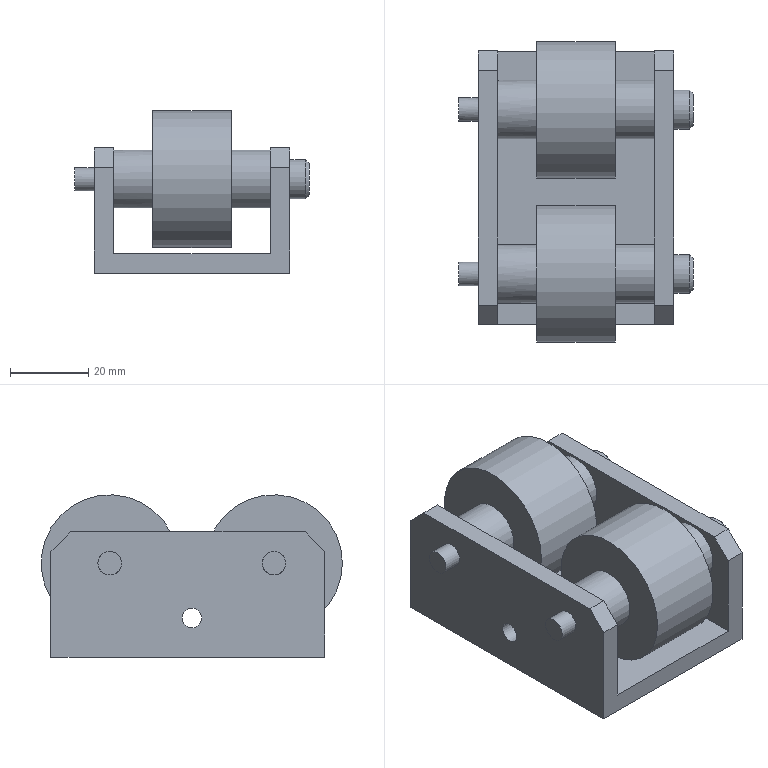Part | NX | features solid 2 | 1 solid | 36 faces | box 60 x 77 x 41.5 mm | volume 82546 mm3 | plane 22 | cylinder 12 | cone 2 | commonest cylinder face diameters 15 x4 5 x2 6 x2 10 x2 35 x2
STEP:
#1=CARTESIAN_POINT('',(200.,655.5,-126.));
#2=VERTEX_POINT('',#1);
#3=CARTESIAN_POINT('',(200.,673.,-126.));
#4=DIRECTION('',(1.,0.,0.));
#5=DIRECTION('',(0.,-1.,0.));
#6=AXIS2_PLACEMENT_3D('',#3,#4,#5);
#7=CIRCLE('',#6,17.5);
#8=EDGE_CURVE('',#2,#2,#7,.T.);
#9=ORIENTED_EDGE('',*,*,#8,.F.);
#10=EDGE_LOOP('',(#9));
#11=FACE_BOUND('',#10,.T.);
#12=CARTESIAN_POINT('',(180.,655.5,-126.));
#13=VERTEX_POINT('',#12);
#14=CARTESIAN_POINT('',(180.,673.,-126.));
#15=DIRECTION('',(1.,0.,0.));
#16=DIRECTION('',(0.,-1.,0.));
#17=AXIS2_PLACEMENT_3D('',#14,#15,#16);
#18=CIRCLE('',#17,17.5);
#19=EDGE_CURVE('',#13,#13,#18,.T.);
#20=ORIENTED_EDGE('',*,*,#19,.T.);
#21=EDGE_LOOP('',(#20));
#22=FACE_BOUND('',#21,.T.);
#23=CARTESIAN_POINT('',(180.,673.,-126.));
#24=DIRECTION('',(1.,0.,0.));
#25=DIRECTION('',(0.,0.,-1.));
#26=AXIS2_PLACEMENT_3D('',#23,#24,#25);
#27=CYLINDRICAL_SURFACE('',#26,17.5);
#28=ADVANCED_FACE('',(#11,#22),#27,.T.);
#29=ORIENTED_EDGE('',*,*,#8,.T.);
#30=EDGE_LOOP('',(#29));
#31=FACE_BOUND('',#30,.T.);
#32=CARTESIAN_POINT('',(200.,665.5,-126.));
#33=VERTEX_POINT('',#32);
#34=CARTESIAN_POINT('',(200.,673.,-126.));
#35=DIRECTION('',(1.,0.,0.));
#36=DIRECTION('',(0.,-1.,0.));
#37=AXIS2_PLACEMENT_3D('',#34,#35,#36);
#38=CIRCLE('',#37,7.5);
#39=EDGE_CURVE('',#33,#33,#38,.T.);
#40=ORIENTED_EDGE('',*,*,#39,.F.);
#41=EDGE_LOOP('',(#40));
#42=FACE_BOUND('',#41,.T.);
#43=CARTESIAN_POINT('',(200.,673.,-126.));
#44=DIRECTION('',(-1.,0.,0.));
#45=DIRECTION('',(0.,0.,1.));
#46=AXIS2_PLACEMENT_3D('',#43,#44,#45);
#47=PLANE('',#46);
#48=ADVANCED_FACE('',(#31,#42),#47,.F.);
#49=ORIENTED_EDGE('',*,*,#19,.F.);
#50=EDGE_LOOP('',(#49));
#51=FACE_BOUND('',#50,.T.);
#52=CARTESIAN_POINT('',(180.,665.5,-126.));
#53=VERTEX_POINT('',#52);
#54=CARTESIAN_POINT('',(180.,673.,-126.));
#55=DIRECTION('',(1.,0.,0.));
#56=DIRECTION('',(0.,-1.,0.));
#57=AXIS2_PLACEMENT_3D('',#54,#55,#56);
#58=CIRCLE('',#57,7.5);
#59=EDGE_CURVE('',#53,#53,#58,.T.);
#60=ORIENTED_EDGE('',*,*,#59,.T.);
#61=EDGE_LOOP('',(#60));
#62=FACE_BOUND('',#61,.T.);
#63=CARTESIAN_POINT('',(180.,673.,-126.));
#64=DIRECTION('',(-1.,0.,0.));
#65=DIRECTION('',(0.,0.,1.));
#66=AXIS2_PLACEMENT_3D('',#63,#64,#65);
#67=PLANE('',#66);
#68=ADVANCED_FACE('',(#51,#62),#67,.T.);
#69=CARTESIAN_POINT('',(220.,673.,-122.));
#70=VERTEX_POINT('',#69);
#71=CARTESIAN_POINT('',(220.,673.,-126.));
#72=DIRECTION('',(1.,0.,0.));
#73=DIRECTION('',(0.,0.,1.));
#74=AXIS2_PLACEMENT_3D('',#71,#72,#73);
#75=CIRCLE('',#74,4.);
#76=EDGE_CURVE('',#70,#70,#75,.F.);
#77=ORIENTED_EDGE('',*,*,#76,.F.);
#78=EDGE_LOOP('',(#77));
#79=FACE_BOUND('',#78,.T.);
#80=CARTESIAN_POINT('',(220.,673.,-126.));
#81=DIRECTION('',(-1.,0.,0.));
#82=DIRECTION('',(0.,0.,1.));
#83=AXIS2_PLACEMENT_3D('',#80,#81,#82);
#84=PLANE('',#83);
#85=ADVANCED_FACE('',(#79),#84,.F.);
#86=CARTESIAN_POINT('',(219.,673.,-121.));
#87=VERTEX_POINT('',#86);
#88=CARTESIAN_POINT('',(219.,673.,-126.));
#89=DIRECTION('',(1.,0.,0.));
#90=DIRECTION('',(0.,0.,1.));
#91=AXIS2_PLACEMENT_3D('',#88,#89,#90);
#92=CIRCLE('',#91,5.);
#93=EDGE_CURVE('',#87,#87,#92,.T.);
#94=ORIENTED_EDGE('',*,*,#93,.T.);
#95=EDGE_LOOP('',(#94));
#96=FACE_BOUND('',#95,.T.);
#97=ORIENTED_EDGE('',*,*,#76,.T.);
#98=EDGE_LOOP('',(#97));
#99=FACE_BOUND('',#98,.T.);
#100=CARTESIAN_POINT('',(219.,673.,-126.));
#101=DIRECTION('',(-1.,0.,0.));
#102=DIRECTION('',(0.,0.,1.));
#103=AXIS2_PLACEMENT_3D('',#100,#101,#102);
#104=CONICAL_SURFACE('',#103,5.,0.7854);
#105=ADVANCED_FACE('',(#96,#99),#104,.T.);
#106=ORIENTED_EDGE('',*,*,#93,.F.);
#107=EDGE_LOOP('',(#106));
#108=FACE_BOUND('',#107,.T.);
#109=CARTESIAN_POINT('',(215.,673.,-131.));
#110=VERTEX_POINT('',#109);
#111=CARTESIAN_POINT('',(215.,673.,-126.));
#112=DIRECTION('',(-1.,0.,0.));
#113=DIRECTION('',(0.,0.,-1.));
#114=AXIS2_PLACEMENT_3D('',#111,#112,#113);
#115=CIRCLE('',#114,5.);
#116=EDGE_CURVE('',#110,#110,#115,.T.);
#117=ORIENTED_EDGE('',*,*,#116,.F.);
#118=EDGE_LOOP('',(#117));
#119=FACE_BOUND('',#118,.T.);
#120=CARTESIAN_POINT('',(220.,673.,-126.));
#121=DIRECTION('',(-1.,0.,0.));
#122=DIRECTION('',(0.,0.,1.));
#123=AXIS2_PLACEMENT_3D('',#120,#121,#122);
#124=CYLINDRICAL_SURFACE('',#123,5.);
#125=ADVANCED_FACE('',(#108,#119),#124,.T.);
#126=ORIENTED_EDGE('',*,*,#59,.F.);
#127=EDGE_LOOP('',(#126));
#128=FACE_BOUND('',#127,.T.);
#129=CARTESIAN_POINT('',(170.,673.,-118.5));
#130=VERTEX_POINT('',#129);
#131=CARTESIAN_POINT('',(170.,673.,-126.));
#132=DIRECTION('',(1.,0.,0.));
#133=DIRECTION('',(0.,0.,1.));
#134=AXIS2_PLACEMENT_3D('',#131,#132,#133);
#135=CIRCLE('',#134,7.5);
#136=EDGE_CURVE('',#130,#130,#135,.F.);
#137=ORIENTED_EDGE('',*,*,#136,.F.);
#138=EDGE_LOOP('',(#137));
#139=FACE_BOUND('',#138,.T.);
#140=CARTESIAN_POINT('',(170.,673.,-126.));
#141=DIRECTION('',(1.,0.,0.));
#142=DIRECTION('',(0.,0.,-1.));
#143=AXIS2_PLACEMENT_3D('',#140,#141,#142);
#144=CYLINDRICAL_SURFACE('',#143,7.5);
#145=ADVANCED_FACE('',(#128,#139),#144,.T.);
#146=CARTESIAN_POINT('',(210.,665.5,-126.));
#147=VERTEX_POINT('',#146);
#148=CARTESIAN_POINT('',(210.,673.,-126.));
#149=DIRECTION('',(1.,0.,0.));
#150=DIRECTION('',(0.,-1.,0.));
#151=AXIS2_PLACEMENT_3D('',#148,#149,#150);
#152=CIRCLE('',#151,7.5);
#153=EDGE_CURVE('',#147,#147,#152,.T.);
#154=ORIENTED_EDGE('',*,*,#153,.F.);
#155=EDGE_LOOP('',(#154));
#156=FACE_BOUND('',#155,.T.);
#157=ORIENTED_EDGE('',*,*,#39,.T.);
#158=EDGE_LOOP('',(#157));
#159=FACE_BOUND('',#158,.T.);
#160=CARTESIAN_POINT('',(210.,673.,-126.));
#161=DIRECTION('',(-1.,0.,0.));
#162=DIRECTION('',(0.,0.,1.));
#163=AXIS2_PLACEMENT_3D('',#160,#161,#162);
#164=CYLINDRICAL_SURFACE('',#163,7.5);
#165=ADVANCED_FACE('',(#156,#159),#164,.T.);
#166=CARTESIAN_POINT('',(210.,730.,-145.));
#167=VERTEX_POINT('',#166);
#168=CARTESIAN_POINT('',(210.,660.,-145.));
#169=VERTEX_POINT('',#168);
#170=CARTESIAN_POINT('',(210.,730.,-145.));
#171=DIRECTION('',(0.,-1.,0.));
#172=VECTOR('',#171,1000.);
#173=LINE('',#170,#172);
#174=EDGE_CURVE('',#167,#169,#173,.T.);
#175=ORIENTED_EDGE('',*,*,#174,.F.);
#176=CARTESIAN_POINT('',(170.,730.,-145.));
#177=VERTEX_POINT('',#176);
#178=CARTESIAN_POINT('',(215.,730.,-145.));
#179=DIRECTION('',(-1.,0.,0.));
#180=VECTOR('',#179,1000.);
#181=LINE('',#178,#180);
#182=EDGE_CURVE('',#167,#177,#181,.T.);
#183=ORIENTED_EDGE('',*,*,#182,.T.);
#184=CARTESIAN_POINT('',(170.,660.,-145.));
#185=VERTEX_POINT('',#184);
#186=CARTESIAN_POINT('',(170.,730.,-145.));
#187=DIRECTION('',(0.,-1.,0.));
#188=VECTOR('',#187,1000.);
#189=LINE('',#186,#188);
#190=EDGE_CURVE('',#177,#185,#189,.T.);
#191=ORIENTED_EDGE('',*,*,#190,.T.);
#192=CARTESIAN_POINT('',(215.,660.,-145.));
#193=DIRECTION('',(-1.,0.,0.));
#194=VECTOR('',#193,1000.);
#195=LINE('',#192,#194);
#196=EDGE_CURVE('',#169,#185,#195,.T.);
#197=ORIENTED_EDGE('',*,*,#196,.F.);
#198=EDGE_LOOP('',(#175,#183,#191,#197));
#199=FACE_BOUND('',#198,.T.);
#200=CARTESIAN_POINT('',(215.,730.,-145.));
#201=DIRECTION('',(0.,0.,-1.));
#202=DIRECTION('',(0.,1.,0.));
#203=AXIS2_PLACEMENT_3D('',#200,#201,#202);
#204=PLANE('',#203);
#205=ADVANCED_FACE('',(#199),#204,.F.);
#206=CARTESIAN_POINT('',(170.,725.,-118.));
#207=VERTEX_POINT('',#206);
#208=CARTESIAN_POINT('',(170.,665.,-118.));
#209=VERTEX_POINT('',#208);
#210=CARTESIAN_POINT('',(170.,730.,-118.));
#211=DIRECTION('',(0.,-1.,0.));
#212=VECTOR('',#211,1000.);
#213=LINE('',#210,#212);
#214=EDGE_CURVE('',#207,#209,#213,.T.);
#215=ORIENTED_EDGE('',*,*,#214,.F.);
#216=CARTESIAN_POINT('',(165.,725.,-118.));
#217=VERTEX_POINT('',#216);
#218=CARTESIAN_POINT('',(165.,725.,-118.));
#219=DIRECTION('',(1.,0.,0.));
#220=VECTOR('',#219,1000.);
#221=LINE('',#218,#220);
#222=EDGE_CURVE('',#217,#207,#221,.T.);
#223=ORIENTED_EDGE('',*,*,#222,.F.);
#224=CARTESIAN_POINT('',(165.,665.,-118.));
#225=VERTEX_POINT('',#224);
#226=CARTESIAN_POINT('',(165.,730.,-118.));
#227=DIRECTION('',(0.,-1.,0.));
#228=VECTOR('',#227,1000.);
#229=LINE('',#226,#228);
#230=EDGE_CURVE('',#217,#225,#229,.T.);
#231=ORIENTED_EDGE('',*,*,#230,.T.);
#232=CARTESIAN_POINT('',(165.,665.,-118.));
#233=DIRECTION('',(-1.,0.,0.));
#234=VECTOR('',#233,1000.);
#235=LINE('',#232,#234);
#236=EDGE_CURVE('',#209,#225,#235,.T.);
#237=ORIENTED_EDGE('',*,*,#236,.F.);
#238=EDGE_LOOP('',(#215,#223,#231,#237));
#239=FACE_BOUND('',#238,.T.);
#240=CARTESIAN_POINT('',(165.,730.,-118.));
#241=DIRECTION('',(0.,0.,1.));
#242=DIRECTION('',(0.,-1.,0.));
#243=AXIS2_PLACEMENT_3D('',#240,#241,#242);
#244=PLANE('',#243);
#245=ADVANCED_FACE('',(#239),#244,.T.);
#246=CARTESIAN_POINT('',(215.,660.,-150.));
#247=VERTEX_POINT('',#246);
#248=CARTESIAN_POINT('',(165.,660.,-150.));
#249=VERTEX_POINT('',#248);
#250=CARTESIAN_POINT('',(215.,660.,-150.));
#251=DIRECTION('',(-1.,0.,0.));
#252=VECTOR('',#251,1000.);
#253=LINE('',#250,#252);
#254=EDGE_CURVE('',#247,#249,#253,.T.);
#255=ORIENTED_EDGE('',*,*,#254,.T.);
#256=CARTESIAN_POINT('',(165.,730.,-150.));
#257=VERTEX_POINT('',#256);
#258=CARTESIAN_POINT('',(165.,730.,-150.));
#259=DIRECTION('',(0.,-1.,0.));
#260=VECTOR('',#259,1000.);
#261=LINE('',#258,#260);
#262=EDGE_CURVE('',#257,#249,#261,.T.);
#263=ORIENTED_EDGE('',*,*,#262,.F.);
#264=CARTESIAN_POINT('',(215.,730.,-150.));
#265=VERTEX_POINT('',#264);
#266=CARTESIAN_POINT('',(215.,730.,-150.));
#267=DIRECTION('',(-1.,0.,0.));
#268=VECTOR('',#267,1000.);
#269=LINE('',#266,#268);
#270=EDGE_CURVE('',#265,#257,#269,.T.);
#271=ORIENTED_EDGE('',*,*,#270,.F.);
#272=CARTESIAN_POINT('',(215.,730.,-150.));
#273=DIRECTION('',(0.,-1.,0.));
#274=VECTOR('',#273,1000.);
#275=LINE('',#272,#274);
#276=EDGE_CURVE('',#265,#247,#275,.T.);
#277=ORIENTED_EDGE('',*,*,#276,.T.);
#278=EDGE_LOOP('',(#255,#263,#271,#277));
#279=FACE_BOUND('',#278,.T.);
#280=CARTESIAN_POINT('',(215.,730.,-150.));
#281=DIRECTION('',(0.,0.,-1.));
#282=DIRECTION('',(0.,1.,0.));
#283=AXIS2_PLACEMENT_3D('',#280,#281,#282);
#284=PLANE('',#283);
#285=ADVANCED_FACE('',(#279),#284,.T.);
#286=CARTESIAN_POINT('',(215.,725.,-118.));
#287=VERTEX_POINT('',#286);
#288=CARTESIAN_POINT('',(215.,665.,-118.));
#289=VERTEX_POINT('',#288);
#290=CARTESIAN_POINT('',(215.,730.,-118.));
#291=DIRECTION('',(0.,-1.,0.));
#292=VECTOR('',#291,1000.);
#293=LINE('',#290,#292);
#294=EDGE_CURVE('',#287,#289,#293,.T.);
#295=ORIENTED_EDGE('',*,*,#294,.F.);
#296=CARTESIAN_POINT('',(210.,725.,-118.));
#297=VERTEX_POINT('',#296);
#298=CARTESIAN_POINT('',(215.,725.,-118.));
#299=DIRECTION('',(-1.,0.,0.));
#300=VECTOR('',#299,1000.);
#301=LINE('',#298,#300);
#302=EDGE_CURVE('',#297,#287,#301,.F.);
#303=ORIENTED_EDGE('',*,*,#302,.F.);
#304=CARTESIAN_POINT('',(210.,665.,-118.));
#305=VERTEX_POINT('',#304);
#306=CARTESIAN_POINT('',(210.,730.,-118.));
#307=DIRECTION('',(0.,-1.,0.));
#308=VECTOR('',#307,1000.);
#309=LINE('',#306,#308);
#310=EDGE_CURVE('',#297,#305,#309,.T.);
#311=ORIENTED_EDGE('',*,*,#310,.T.);
#312=CARTESIAN_POINT('',(210.,665.,-118.));
#313=DIRECTION('',(1.,0.,0.));
#314=VECTOR('',#313,1000.);
#315=LINE('',#312,#314);
#316=EDGE_CURVE('',#289,#305,#315,.F.);
#317=ORIENTED_EDGE('',*,*,#316,.F.);
#318=EDGE_LOOP('',(#295,#303,#311,#317));
#319=FACE_BOUND('',#318,.T.);
#320=CARTESIAN_POINT('',(215.,730.,-118.));
#321=DIRECTION('',(0.,0.,-1.));
#322=DIRECTION('',(0.,-1.,0.));
#323=AXIS2_PLACEMENT_3D('',#320,#321,#322);
#324=PLANE('',#323);
#325=ADVANCED_FACE('',(#319),#324,.F.);
#326=CARTESIAN_POINT('',(215.,660.,-123.));
#327=VERTEX_POINT('',#326);
#328=CARTESIAN_POINT('',(215.,660.,-118.));
#329=DIRECTION('',(0.,0.,-1.));
#330=VECTOR('',#329,1000.);
#331=LINE('',#328,#330);
#332=EDGE_CURVE('',#327,#247,#331,.T.);
#333=ORIENTED_EDGE('',*,*,#332,.T.);
#334=ORIENTED_EDGE('',*,*,#276,.F.);
#335=CARTESIAN_POINT('',(215.,730.,-123.));
#336=VERTEX_POINT('',#335);
#337=CARTESIAN_POINT('',(215.,730.,-118.));
#338=DIRECTION('',(0.,0.,-1.));
#339=VECTOR('',#338,1000.);
#340=LINE('',#337,#339);
#341=EDGE_CURVE('',#336,#265,#340,.T.);
#342=ORIENTED_EDGE('',*,*,#341,.F.);
#343=CARTESIAN_POINT('',(215.,727.5,-120.5));
#344=DIRECTION('',(0.,0.7071,-0.7071));
#345=VECTOR('',#344,1000.);
#346=LINE('',#343,#345);
#347=EDGE_CURVE('',#287,#336,#346,.T.);
#348=ORIENTED_EDGE('',*,*,#347,.F.);
#349=ORIENTED_EDGE('',*,*,#294,.T.);
#350=CARTESIAN_POINT('',(215.,697.5,-85.5));
#351=DIRECTION('',(0.,-0.7071,-0.7071));
#352=VECTOR('',#351,1000.);
#353=LINE('',#350,#352);
#354=EDGE_CURVE('',#327,#289,#353,.F.);
#355=ORIENTED_EDGE('',*,*,#354,.F.);
#356=EDGE_LOOP('',(#333,#334,#342,#348,#349,#355));
#357=FACE_BOUND('',#356,.T.);
#358=ORIENTED_EDGE('',*,*,#116,.T.);
#359=EDGE_LOOP('',(#358));
#360=FACE_BOUND('',#359,.T.);
#361=CARTESIAN_POINT('',(215.,715.,-131.));
#362=VERTEX_POINT('',#361);
#363=CARTESIAN_POINT('',(215.,715.,-126.));
#364=DIRECTION('',(-1.,0.,0.));
#365=DIRECTION('',(0.,0.,-1.));
#366=AXIS2_PLACEMENT_3D('',#363,#364,#365);
#367=CIRCLE('',#366,5.);
#368=EDGE_CURVE('',#362,#362,#367,.T.);
#369=ORIENTED_EDGE('',*,*,#368,.T.);
#370=EDGE_LOOP('',(#369));
#371=FACE_BOUND('',#370,.T.);
#372=CARTESIAN_POINT('',(215.,694.,-142.5));
#373=VERTEX_POINT('',#372);
#374=CARTESIAN_POINT('',(215.,694.,-140.));
#375=DIRECTION('',(-1.,0.,0.));
#376=DIRECTION('',(0.,0.,-1.));
#377=AXIS2_PLACEMENT_3D('',#374,#375,#376);
#378=CIRCLE('',#377,2.5);
#379=EDGE_CURVE('',#373,#373,#378,.F.);
#380=ORIENTED_EDGE('',*,*,#379,.F.);
#381=EDGE_LOOP('',(#380));
#382=FACE_BOUND('',#381,.T.);
#383=CARTESIAN_POINT('',(215.,730.,-118.));
#384=DIRECTION('',(1.,0.,0.));
#385=DIRECTION('',(0.,0.,-1.));
#386=AXIS2_PLACEMENT_3D('',#383,#384,#385);
#387=PLANE('',#386);
#388=ADVANCED_FACE('',(#357,#360,#371,#382),#387,.T.);
#389=ORIENTED_EDGE('',*,*,#230,.F.);
#390=CARTESIAN_POINT('',(165.,730.,-123.));
#391=VERTEX_POINT('',#390);
#392=CARTESIAN_POINT('',(165.,743.5,-136.5));
#393=DIRECTION('',(0.,0.7071,-0.7071));
#394=VECTOR('',#393,1000.);
#395=LINE('',#392,#394);
#396=EDGE_CURVE('',#391,#217,#395,.F.);
#397=ORIENTED_EDGE('',*,*,#396,.F.);
#398=CARTESIAN_POINT('',(165.,730.,-150.));
#399=DIRECTION('',(0.,0.,1.));
#400=VECTOR('',#399,1000.);
#401=LINE('',#398,#400);
#402=EDGE_CURVE('',#257,#391,#401,.T.);
#403=ORIENTED_EDGE('',*,*,#402,.F.);
#404=ORIENTED_EDGE('',*,*,#262,.T.);
#405=CARTESIAN_POINT('',(165.,660.,-123.));
#406=VERTEX_POINT('',#405);
#407=CARTESIAN_POINT('',(165.,660.,-150.));
#408=DIRECTION('',(0.,0.,1.));
#409=VECTOR('',#408,1000.);
#410=LINE('',#407,#409);
#411=EDGE_CURVE('',#249,#406,#410,.T.);
#412=ORIENTED_EDGE('',*,*,#411,.T.);
#413=CARTESIAN_POINT('',(165.,681.5,-101.5));
#414=DIRECTION('',(0.,-0.7071,-0.7071));
#415=VECTOR('',#414,1000.);
#416=LINE('',#413,#415);
#417=EDGE_CURVE('',#225,#406,#416,.T.);
#418=ORIENTED_EDGE('',*,*,#417,.F.);
#419=EDGE_LOOP('',(#389,#397,#403,#404,#412,#418));
#420=FACE_BOUND('',#419,.T.);
#421=CARTESIAN_POINT('',(165.,673.,-123.));
#422=VERTEX_POINT('',#421);
#423=CARTESIAN_POINT('',(165.,673.,-126.));
#424=DIRECTION('',(1.,0.,0.));
#425=DIRECTION('',(0.,0.,1.));
#426=AXIS2_PLACEMENT_3D('',#423,#424,#425);
#427=CIRCLE('',#426,3.);
#428=EDGE_CURVE('',#422,#422,#427,.F.);
#429=ORIENTED_EDGE('',*,*,#428,.F.);
#430=EDGE_LOOP('',(#429));
#431=FACE_BOUND('',#430,.T.);
#432=CARTESIAN_POINT('',(165.,715.,-123.));
#433=VERTEX_POINT('',#432);
#434=CARTESIAN_POINT('',(165.,715.,-126.));
#435=DIRECTION('',(1.,0.,0.));
#436=DIRECTION('',(0.,0.,1.));
#437=AXIS2_PLACEMENT_3D('',#434,#435,#436);
#438=CIRCLE('',#437,3.);
#439=EDGE_CURVE('',#433,#433,#438,.F.);
#440=ORIENTED_EDGE('',*,*,#439,.F.);
#441=EDGE_LOOP('',(#440));
#442=FACE_BOUND('',#441,.T.);
#443=CARTESIAN_POINT('',(165.,694.,-137.5));
#444=VERTEX_POINT('',#443);
#445=CARTESIAN_POINT('',(165.,694.,-140.));
#446=DIRECTION('',(1.,0.,0.));
#447=DIRECTION('',(0.,0.,1.));
#448=AXIS2_PLACEMENT_3D('',#445,#446,#447);
#449=CIRCLE('',#448,2.5);
#450=EDGE_CURVE('',#444,#444,#449,.F.);
#451=ORIENTED_EDGE('',*,*,#450,.F.);
#452=EDGE_LOOP('',(#451));
#453=FACE_BOUND('',#452,.T.);
#454=CARTESIAN_POINT('',(165.,730.,-150.));
#455=DIRECTION('',(-1.,0.,0.));
#456=DIRECTION('',(0.,0.,1.));
#457=AXIS2_PLACEMENT_3D('',#454,#455,#456);
#458=PLANE('',#457);
#459=ADVANCED_FACE('',(#420,#431,#442,#453),#458,.T.);
#460=ORIENTED_EDGE('',*,*,#310,.F.);
#461=CARTESIAN_POINT('',(210.,730.,-123.));
#462=VERTEX_POINT('',#461);
#463=CARTESIAN_POINT('',(210.,730.,-123.));
#464=DIRECTION('',(0.,-0.7071,0.7071));
#465=VECTOR('',#464,1000.);
#466=LINE('',#463,#465);
#467=EDGE_CURVE('',#462,#297,#466,.T.);
#468=ORIENTED_EDGE('',*,*,#467,.F.);
#469=CARTESIAN_POINT('',(210.,730.,-118.));
#470=DIRECTION('',(0.,0.,-1.));
#471=VECTOR('',#470,1000.);
#472=LINE('',#469,#471);
#473=EDGE_CURVE('',#462,#167,#472,.T.);
#474=ORIENTED_EDGE('',*,*,#473,.T.);
#475=ORIENTED_EDGE('',*,*,#174,.T.);
#476=CARTESIAN_POINT('',(210.,660.,-123.));
#477=VERTEX_POINT('',#476);
#478=CARTESIAN_POINT('',(210.,660.,-118.));
#479=DIRECTION('',(0.,0.,-1.));
#480=VECTOR('',#479,1000.);
#481=LINE('',#478,#480);
#482=EDGE_CURVE('',#477,#169,#481,.T.);
#483=ORIENTED_EDGE('',*,*,#482,.F.);
#484=CARTESIAN_POINT('',(210.,660.,-123.));
#485=DIRECTION('',(0.,0.7071,0.7071));
#486=VECTOR('',#485,1000.);
#487=LINE('',#484,#486);
#488=EDGE_CURVE('',#305,#477,#487,.F.);
#489=ORIENTED_EDGE('',*,*,#488,.F.);
#490=EDGE_LOOP('',(#460,#468,#474,#475,#483,#489));
#491=FACE_BOUND('',#490,.T.);
#492=ORIENTED_EDGE('',*,*,#153,.T.);
#493=EDGE_LOOP('',(#492));
#494=FACE_BOUND('',#493,.T.);
#495=CARTESIAN_POINT('',(210.,707.5,-126.));
#496=VERTEX_POINT('',#495);
#497=CARTESIAN_POINT('',(210.,715.,-126.));
#498=DIRECTION('',(1.,0.,0.));
#499=DIRECTION('',(0.,-1.,0.));
#500=AXIS2_PLACEMENT_3D('',#497,#498,#499);
#501=CIRCLE('',#500,7.5);
#502=EDGE_CURVE('',#496,#496,#501,.T.);
#503=ORIENTED_EDGE('',*,*,#502,.T.);
#504=EDGE_LOOP('',(#503));
#505=FACE_BOUND('',#504,.T.);
#506=CARTESIAN_POINT('',(210.,694.,-142.5));
#507=VERTEX_POINT('',#506);
#508=CARTESIAN_POINT('',(210.,694.,-140.));
#509=DIRECTION('',(-1.,0.,0.));
#510=DIRECTION('',(0.,0.,-1.));
#511=AXIS2_PLACEMENT_3D('',#508,#509,#510);
#512=CIRCLE('',#511,2.5);
#513=EDGE_CURVE('',#507,#507,#512,.F.);
#514=ORIENTED_EDGE('',*,*,#513,.T.);
#515=EDGE_LOOP('',(#514));
#516=FACE_BOUND('',#515,.T.);
#517=CARTESIAN_POINT('',(210.,730.,-118.));
#518=DIRECTION('',(1.,0.,0.));
#519=DIRECTION('',(0.,0.,-1.));
#520=AXIS2_PLACEMENT_3D('',#517,#518,#519);
#521=PLANE('',#520);
#522=ADVANCED_FACE('',(#491,#494,#505,#516),#521,.F.);
#523=CARTESIAN_POINT('',(170.,660.,-123.));
#524=VERTEX_POINT('',#523);
#525=CARTESIAN_POINT('',(170.,660.,-150.));
#526=DIRECTION('',(0.,0.,1.));
#527=VECTOR('',#526,1000.);
#528=LINE('',#525,#527);
#529=EDGE_CURVE('',#185,#524,#528,.T.);
#530=ORIENTED_EDGE('',*,*,#529,.F.);
#531=ORIENTED_EDGE('',*,*,#190,.F.);
#532=CARTESIAN_POINT('',(170.,730.,-123.));
#533=VERTEX_POINT('',#532);
#534=CARTESIAN_POINT('',(170.,730.,-150.));
#535=DIRECTION('',(0.,0.,1.));
#536=VECTOR('',#535,1000.);
#537=LINE('',#534,#536);
#538=EDGE_CURVE('',#177,#533,#537,.T.);
#539=ORIENTED_EDGE('',*,*,#538,.T.);
#540=CARTESIAN_POINT('',(170.,725.,-118.));
#541=DIRECTION('',(0.,-0.7071,0.7071));
#542=VECTOR('',#541,1000.);
#543=LINE('',#540,#542);
#544=EDGE_CURVE('',#207,#533,#543,.F.);
#545=ORIENTED_EDGE('',*,*,#544,.F.);
#546=ORIENTED_EDGE('',*,*,#214,.T.);
#547=CARTESIAN_POINT('',(170.,660.,-123.));
#548=DIRECTION('',(0.,0.7071,0.7071));
#549=VECTOR('',#548,1000.);
#550=LINE('',#547,#549);
#551=EDGE_CURVE('',#524,#209,#550,.T.);
#552=ORIENTED_EDGE('',*,*,#551,.F.);
#553=EDGE_LOOP('',(#530,#531,#539,#545,#546,#552));
#554=FACE_BOUND('',#553,.T.);
#555=ORIENTED_EDGE('',*,*,#136,.T.);
#556=EDGE_LOOP('',(#555));
#557=FACE_BOUND('',#556,.T.);
#558=CARTESIAN_POINT('',(170.,715.,-118.5));
#559=VERTEX_POINT('',#558);
#560=CARTESIAN_POINT('',(170.,715.,-126.));
#561=DIRECTION('',(1.,0.,0.));
#562=DIRECTION('',(0.,0.,1.));
#563=AXIS2_PLACEMENT_3D('',#560,#561,#562);
#564=CIRCLE('',#563,7.5);
#565=EDGE_CURVE('',#559,#559,#564,.F.);
#566=ORIENTED_EDGE('',*,*,#565,.T.);
#567=EDGE_LOOP('',(#566));
#568=FACE_BOUND('',#567,.T.);
#569=CARTESIAN_POINT('',(170.,694.,-137.5));
#570=VERTEX_POINT('',#569);
#571=CARTESIAN_POINT('',(170.,694.,-140.));
#572=DIRECTION('',(1.,0.,0.));
#573=DIRECTION('',(0.,0.,1.));
#574=AXIS2_PLACEMENT_3D('',#571,#572,#573);
#575=CIRCLE('',#574,2.5);
#576=EDGE_CURVE('',#570,#570,#575,.F.);
#577=ORIENTED_EDGE('',*,*,#576,.T.);
#578=EDGE_LOOP('',(#577));
#579=FACE_BOUND('',#578,.T.);
#580=CARTESIAN_POINT('',(170.,730.,-150.));
#581=DIRECTION('',(-1.,0.,0.));
#582=DIRECTION('',(0.,0.,1.));
#583=AXIS2_PLACEMENT_3D('',#580,#581,#582);
#584=PLANE('',#583);
#585=ADVANCED_FACE('',(#554,#557,#568,#579),#584,.F.);
#586=ORIENTED_EDGE('',*,*,#482,.T.);
#587=ORIENTED_EDGE('',*,*,#196,.T.);
#588=ORIENTED_EDGE('',*,*,#529,.T.);
#589=CARTESIAN_POINT('',(170.,660.,-123.));
#590=DIRECTION('',(1.,0.,0.));
#591=VECTOR('',#590,1000.);
#592=LINE('',#589,#591);
#593=EDGE_CURVE('',#406,#524,#592,.T.);
#594=ORIENTED_EDGE('',*,*,#593,.F.);
#595=ORIENTED_EDGE('',*,*,#411,.F.);
#596=ORIENTED_EDGE('',*,*,#254,.F.);
#597=ORIENTED_EDGE('',*,*,#332,.F.);
#598=CARTESIAN_POINT('',(215.,660.,-123.));
#599=DIRECTION('',(1.,0.,0.));
#600=VECTOR('',#599,1000.);
#601=LINE('',#598,#600);
#602=EDGE_CURVE('',#477,#327,#601,.T.);
#603=ORIENTED_EDGE('',*,*,#602,.F.);
#604=EDGE_LOOP('',(#586,#587,#588,#594,#595,#596,#597,#603));
#605=FACE_BOUND('',#604,.T.);
#606=CARTESIAN_POINT('',(192.5,660.,-129.38));
#607=DIRECTION('',(0.,1.,0.));
#608=DIRECTION('',(0.,0.,1.));
#609=AXIS2_PLACEMENT_3D('',#606,#607,#608);
#610=PLANE('',#609);
#611=ADVANCED_FACE('',(#605),#610,.F.);
#612=CARTESIAN_POINT('',(180.,697.5,-126.));
#613=VERTEX_POINT('',#612);
#614=CARTESIAN_POINT('',(180.,715.,-126.));
#615=DIRECTION('',(1.,0.,0.));
#616=DIRECTION('',(0.,-1.,0.));
#617=AXIS2_PLACEMENT_3D('',#614,#615,#616);
#618=CIRCLE('',#617,17.5);
#619=EDGE_CURVE('',#613,#613,#618,.T.);
#620=ORIENTED_EDGE('',*,*,#619,.T.);
#621=EDGE_LOOP('',(#620));
#622=FACE_BOUND('',#621,.T.);
#623=CARTESIAN_POINT('',(200.,697.5,-126.));
#624=VERTEX_POINT('',#623);
#625=CARTESIAN_POINT('',(200.,715.,-126.));
#626=DIRECTION('',(1.,0.,0.));
#627=DIRECTION('',(0.,-1.,0.));
#628=AXIS2_PLACEMENT_3D('',#625,#626,#627);
#629=CIRCLE('',#628,17.5);
#630=EDGE_CURVE('',#624,#624,#629,.T.);
#631=ORIENTED_EDGE('',*,*,#630,.F.);
#632=EDGE_LOOP('',(#631));
#633=FACE_BOUND('',#632,.T.);
#634=CARTESIAN_POINT('',(180.,715.,-126.));
#635=DIRECTION('',(1.,0.,0.));
#636=DIRECTION('',(0.,0.,-1.));
#637=AXIS2_PLACEMENT_3D('',#634,#635,#636);
#638=CYLINDRICAL_SURFACE('',#637,17.5);
#639=ADVANCED_FACE('',(#622,#633),#638,.T.);
#640=CARTESIAN_POINT('',(220.,715.,-122.));
#641=VERTEX_POINT('',#640);
#642=CARTESIAN_POINT('',(220.,715.,-126.));
#643=DIRECTION('',(1.,0.,0.));
#644=DIRECTION('',(0.,0.,1.));
#645=AXIS2_PLACEMENT_3D('',#642,#643,#644);
#646=CIRCLE('',#645,4.);
#647=EDGE_CURVE('',#641,#641,#646,.F.);
#648=ORIENTED_EDGE('',*,*,#647,.F.);
#649=EDGE_LOOP('',(#648));
#650=FACE_BOUND('',#649,.T.);
#651=CARTESIAN_POINT('',(220.,715.,-126.));
#652=DIRECTION('',(-1.,0.,0.));
#653=DIRECTION('',(0.,0.,1.));
#654=AXIS2_PLACEMENT_3D('',#651,#652,#653);
#655=PLANE('',#654);
#656=ADVANCED_FACE('',(#650),#655,.F.);
#657=ORIENTED_EDGE('',*,*,#619,.F.);
#658=EDGE_LOOP('',(#657));
#659=FACE_BOUND('',#658,.T.);
#660=CARTESIAN_POINT('',(180.,707.5,-126.));
#661=VERTEX_POINT('',#660);
#662=CARTESIAN_POINT('',(180.,715.,-126.));
#663=DIRECTION('',(1.,0.,0.));
#664=DIRECTION('',(0.,-1.,0.));
#665=AXIS2_PLACEMENT_3D('',#662,#663,#664);
#666=CIRCLE('',#665,7.5);
#667=EDGE_CURVE('',#661,#661,#666,.T.);
#668=ORIENTED_EDGE('',*,*,#667,.T.);
#669=EDGE_LOOP('',(#668));
#670=FACE_BOUND('',#669,.T.);
#671=CARTESIAN_POINT('',(180.,715.,-126.));
#672=DIRECTION('',(-1.,0.,0.));
#673=DIRECTION('',(0.,0.,1.));
#674=AXIS2_PLACEMENT_3D('',#671,#672,#673);
#675=PLANE('',#674);
#676=ADVANCED_FACE('',(#659,#670),#675,.T.);
#677=CARTESIAN_POINT('',(200.,707.5,-126.));
#678=VERTEX_POINT('',#677);
#679=CARTESIAN_POINT('',(200.,715.,-126.));
#680=DIRECTION('',(1.,0.,0.));
#681=DIRECTION('',(0.,-1.,0.));
#682=AXIS2_PLACEMENT_3D('',#679,#680,#681);
#683=CIRCLE('',#682,7.5);
#684=EDGE_CURVE('',#678,#678,#683,.T.);
#685=ORIENTED_EDGE('',*,*,#684,.F.);
#686=EDGE_LOOP('',(#685));
#687=FACE_BOUND('',#686,.T.);
#688=ORIENTED_EDGE('',*,*,#630,.T.);
#689=EDGE_LOOP('',(#688));
#690=FACE_BOUND('',#689,.T.);
#691=CARTESIAN_POINT('',(200.,715.,-126.));
#692=DIRECTION('',(-1.,0.,0.));
#693=DIRECTION('',(0.,0.,1.));
#694=AXIS2_PLACEMENT_3D('',#691,#692,#693);
#695=PLANE('',#694);
#696=ADVANCED_FACE('',(#687,#690),#695,.F.);
#697=CARTESIAN_POINT('',(160.,712.,-126.));
#698=VERTEX_POINT('',#697);
#699=CARTESIAN_POINT('',(160.,715.,-126.));
#700=DIRECTION('',(1.,0.,0.));
#701=DIRECTION('',(0.,-1.,0.));
#702=AXIS2_PLACEMENT_3D('',#699,#700,#701);
#703=CIRCLE('',#702,3.);
#704=EDGE_CURVE('',#698,#698,#703,.T.);
#705=ORIENTED_EDGE('',*,*,#704,.F.);
#706=EDGE_LOOP('',(#705));
#707=FACE_BOUND('',#706,.T.);
#708=CARTESIAN_POINT('',(160.,715.,-126.));
#709=DIRECTION('',(-1.,0.,0.));
#710=DIRECTION('',(0.,0.,1.));
#711=AXIS2_PLACEMENT_3D('',#708,#709,#710);
#712=PLANE('',#711);
#713=ADVANCED_FACE('',(#707),#712,.T.);
#714=CARTESIAN_POINT('',(160.,670.,-126.));
#715=VERTEX_POINT('',#714);
#716=CARTESIAN_POINT('',(160.,673.,-126.));
#717=DIRECTION('',(1.,0.,0.));
#718=DIRECTION('',(0.,-1.,0.));
#719=AXIS2_PLACEMENT_3D('',#716,#717,#718);
#720=CIRCLE('',#719,3.);
#721=EDGE_CURVE('',#715,#715,#720,.T.);
#722=ORIENTED_EDGE('',*,*,#721,.F.);
#723=EDGE_LOOP('',(#722));
#724=FACE_BOUND('',#723,.T.);
#725=CARTESIAN_POINT('',(160.,673.,-126.));
#726=DIRECTION('',(-1.,0.,0.));
#727=DIRECTION('',(0.,0.,1.));
#728=AXIS2_PLACEMENT_3D('',#725,#726,#727);
#729=PLANE('',#728);
#730=ADVANCED_FACE('',(#724),#729,.T.);
#731=ORIENTED_EDGE('',*,*,#647,.T.);
#732=EDGE_LOOP('',(#731));
#733=FACE_BOUND('',#732,.T.);
#734=CARTESIAN_POINT('',(219.,715.,-121.));
#735=VERTEX_POINT('',#734);
#736=CARTESIAN_POINT('',(219.,715.,-126.));
#737=DIRECTION('',(1.,0.,0.));
#738=DIRECTION('',(0.,0.,1.));
#739=AXIS2_PLACEMENT_3D('',#736,#737,#738);
#740=CIRCLE('',#739,5.);
#741=EDGE_CURVE('',#735,#735,#740,.T.);
#742=ORIENTED_EDGE('',*,*,#741,.T.);
#743=EDGE_LOOP('',(#742));
#744=FACE_BOUND('',#743,.T.);
#745=CARTESIAN_POINT('',(219.,715.,-126.));
#746=DIRECTION('',(-1.,0.,0.));
#747=DIRECTION('',(0.,0.,1.));
#748=AXIS2_PLACEMENT_3D('',#745,#746,#747);
#749=CONICAL_SURFACE('',#748,5.,0.7854);
#750=ADVANCED_FACE('',(#733,#744),#749,.T.);
#751=ORIENTED_EDGE('',*,*,#565,.F.);
#752=EDGE_LOOP('',(#751));
#753=FACE_BOUND('',#752,.T.);
#754=ORIENTED_EDGE('',*,*,#667,.F.);
#755=EDGE_LOOP('',(#754));
#756=FACE_BOUND('',#755,.T.);
#757=CARTESIAN_POINT('',(170.,715.,-126.));
#758=DIRECTION('',(1.,0.,0.));
#759=DIRECTION('',(0.,0.,-1.));
#760=AXIS2_PLACEMENT_3D('',#757,#758,#759);
#761=CYLINDRICAL_SURFACE('',#760,7.5);
#762=ADVANCED_FACE('',(#753,#756),#761,.T.);
#763=ORIENTED_EDGE('',*,*,#502,.F.);
#764=EDGE_LOOP('',(#763));
#765=FACE_BOUND('',#764,.T.);
#766=ORIENTED_EDGE('',*,*,#684,.T.);
#767=EDGE_LOOP('',(#766));
#768=FACE_BOUND('',#767,.T.);
#769=CARTESIAN_POINT('',(210.,715.,-126.));
#770=DIRECTION('',(-1.,0.,0.));
#771=DIRECTION('',(0.,0.,1.));
#772=AXIS2_PLACEMENT_3D('',#769,#770,#771);
#773=CYLINDRICAL_SURFACE('',#772,7.5);
#774=ADVANCED_FACE('',(#765,#768),#773,.T.);
#775=ORIENTED_EDGE('',*,*,#450,.T.);
#776=EDGE_LOOP('',(#775));
#777=FACE_BOUND('',#776,.T.);
#778=ORIENTED_EDGE('',*,*,#576,.F.);
#779=EDGE_LOOP('',(#778));
#780=FACE_BOUND('',#779,.T.);
#781=CARTESIAN_POINT('',(160.,694.,-140.));
#782=DIRECTION('',(1.,0.,0.));
#783=DIRECTION('',(0.,0.,-1.));
#784=AXIS2_PLACEMENT_3D('',#781,#782,#783);
#785=CYLINDRICAL_SURFACE('',#784,2.5);
#786=ADVANCED_FACE('',(#777,#780),#785,.F.);
#787=ORIENTED_EDGE('',*,*,#439,.T.);
#788=EDGE_LOOP('',(#787));
#789=FACE_BOUND('',#788,.T.);
#790=ORIENTED_EDGE('',*,*,#704,.T.);
#791=EDGE_LOOP('',(#790));
#792=FACE_BOUND('',#791,.T.);
#793=CARTESIAN_POINT('',(160.,715.,-126.));
#794=DIRECTION('',(1.,0.,0.));
#795=DIRECTION('',(0.,0.,-1.));
#796=AXIS2_PLACEMENT_3D('',#793,#794,#795);
#797=CYLINDRICAL_SURFACE('',#796,3.);
#798=ADVANCED_FACE('',(#789,#792),#797,.T.);
#799=ORIENTED_EDGE('',*,*,#428,.T.);
#800=EDGE_LOOP('',(#799));
#801=FACE_BOUND('',#800,.T.);
#802=ORIENTED_EDGE('',*,*,#721,.T.);
#803=EDGE_LOOP('',(#802));
#804=FACE_BOUND('',#803,.T.);
#805=CARTESIAN_POINT('',(160.,673.,-126.));
#806=DIRECTION('',(1.,0.,0.));
#807=DIRECTION('',(0.,0.,-1.));
#808=AXIS2_PLACEMENT_3D('',#805,#806,#807);
#809=CYLINDRICAL_SURFACE('',#808,3.);
#810=ADVANCED_FACE('',(#801,#804),#809,.T.);
#811=ORIENTED_EDGE('',*,*,#379,.T.);
#812=EDGE_LOOP('',(#811));
#813=FACE_BOUND('',#812,.T.);
#814=ORIENTED_EDGE('',*,*,#513,.F.);
#815=EDGE_LOOP('',(#814));
#816=FACE_BOUND('',#815,.T.);
#817=CARTESIAN_POINT('',(160.,694.,-140.));
#818=DIRECTION('',(1.,0.,0.));
#819=DIRECTION('',(0.,0.,-1.));
#820=AXIS2_PLACEMENT_3D('',#817,#818,#819);
#821=CYLINDRICAL_SURFACE('',#820,2.5);
#822=ADVANCED_FACE('',(#813,#816),#821,.F.);
#823=ORIENTED_EDGE('',*,*,#741,.F.);
#824=EDGE_LOOP('',(#823));
#825=FACE_BOUND('',#824,.T.);
#826=ORIENTED_EDGE('',*,*,#368,.F.);
#827=EDGE_LOOP('',(#826));
#828=FACE_BOUND('',#827,.T.);
#829=CARTESIAN_POINT('',(220.,715.,-126.));
#830=DIRECTION('',(-1.,0.,0.));
#831=DIRECTION('',(0.,0.,1.));
#832=AXIS2_PLACEMENT_3D('',#829,#830,#831);
#833=CYLINDRICAL_SURFACE('',#832,5.);
#834=ADVANCED_FACE('',(#825,#828),#833,.T.);
#835=ORIENTED_EDGE('',*,*,#538,.F.);
#836=ORIENTED_EDGE('',*,*,#182,.F.);
#837=ORIENTED_EDGE('',*,*,#473,.F.);
#838=CARTESIAN_POINT('',(215.,730.,-123.));
#839=DIRECTION('',(-1.,0.,0.));
#840=VECTOR('',#839,1000.);
#841=LINE('',#838,#840);
#842=EDGE_CURVE('',#336,#462,#841,.T.);
#843=ORIENTED_EDGE('',*,*,#842,.F.);
#844=ORIENTED_EDGE('',*,*,#341,.T.);
#845=ORIENTED_EDGE('',*,*,#270,.T.);
#846=ORIENTED_EDGE('',*,*,#402,.T.);
#847=CARTESIAN_POINT('',(215.,730.,-123.));
#848=DIRECTION('',(-1.,0.,0.));
#849=VECTOR('',#848,1000.);
#850=LINE('',#847,#849);
#851=EDGE_CURVE('',#533,#391,#850,.T.);
#852=ORIENTED_EDGE('',*,*,#851,.F.);
#853=EDGE_LOOP('',(#835,#836,#837,#843,#844,#845,#846,#852));
#854=FACE_BOUND('',#853,.T.);
#855=CARTESIAN_POINT('',(215.,730.,-118.));
#856=DIRECTION('',(0.,1.,0.));
#857=DIRECTION('',(0.,0.,-1.));
#858=AXIS2_PLACEMENT_3D('',#855,#856,#857);
#859=PLANE('',#858);
#860=ADVANCED_FACE('',(#854),#859,.T.);
#861=ORIENTED_EDGE('',*,*,#488,.T.);
#862=ORIENTED_EDGE('',*,*,#602,.T.);
#863=ORIENTED_EDGE('',*,*,#354,.T.);
#864=ORIENTED_EDGE('',*,*,#316,.T.);
#865=EDGE_LOOP('',(#861,#862,#863,#864));
#866=FACE_BOUND('',#865,.T.);
#867=CARTESIAN_POINT('',(192.5,660.,-123.));
#868=DIRECTION('',(0.,0.7071,-0.7071));
#869=DIRECTION('',(0.,0.7071,0.7071));
#870=AXIS2_PLACEMENT_3D('',#867,#868,#869);
#871=PLANE('',#870);
#872=ADVANCED_FACE('',(#866),#871,.F.);
#873=ORIENTED_EDGE('',*,*,#417,.T.);
#874=ORIENTED_EDGE('',*,*,#593,.T.);
#875=ORIENTED_EDGE('',*,*,#551,.T.);
#876=ORIENTED_EDGE('',*,*,#236,.T.);
#877=EDGE_LOOP('',(#873,#874,#875,#876));
#878=FACE_BOUND('',#877,.T.);
#879=CARTESIAN_POINT('',(192.5,660.,-123.));
#880=DIRECTION('',(0.,-0.7071,0.7071));
#881=DIRECTION('',(0.,-0.7071,-0.7071));
#882=AXIS2_PLACEMENT_3D('',#879,#880,#881);
#883=PLANE('',#882);
#884=ADVANCED_FACE('',(#878),#883,.T.);
#885=ORIENTED_EDGE('',*,*,#396,.T.);
#886=ORIENTED_EDGE('',*,*,#222,.T.);
#887=ORIENTED_EDGE('',*,*,#544,.T.);
#888=ORIENTED_EDGE('',*,*,#851,.T.);
#889=EDGE_LOOP('',(#885,#886,#887,#888));
#890=FACE_BOUND('',#889,.T.);
#891=CARTESIAN_POINT('',(165.,725.,-118.));
#892=DIRECTION('',(0.,-0.7071,-0.7071));
#893=DIRECTION('',(0.,0.7071,-0.7071));
#894=AXIS2_PLACEMENT_3D('',#891,#892,#893);
#895=PLANE('',#894);
#896=ADVANCED_FACE('',(#890),#895,.F.);
#897=ORIENTED_EDGE('',*,*,#347,.T.);
#898=ORIENTED_EDGE('',*,*,#842,.T.);
#899=ORIENTED_EDGE('',*,*,#467,.T.);
#900=ORIENTED_EDGE('',*,*,#302,.T.);
#901=EDGE_LOOP('',(#897,#898,#899,#900));
#902=FACE_BOUND('',#901,.T.);
#903=CARTESIAN_POINT('',(215.,730.,-123.));
#904=DIRECTION('',(0.,0.7071,0.7071));
#905=DIRECTION('',(0.,-0.7071,0.7071));
#906=AXIS2_PLACEMENT_3D('',#903,#904,#905);
#907=PLANE('',#906);
#908=ADVANCED_FACE('',(#902),#907,.T.);
#909=CLOSED_SHELL('',(#28,#48,#68,#85,#105,#125,#145,#165,#205,#245,#285,#325,#388,#459,#522,#585,#611,#639,#656,#676,#696,#713,#730,#750,#762,#774,#786,#798,#810,#822,#834,#860,#872,#884,#896,#908));
#910=MANIFOLD_SOLID_BREP('',#909);
#911=(LENGTH_UNIT()NAMED_UNIT(*)SI_UNIT(.MILLI.,.METRE.));
#912=UNCERTAINTY_MEASURE_WITH_UNIT(LENGTH_MEASURE(0.00001),#911,'','');
#913=(NAMED_UNIT(*)PLANE_ANGLE_UNIT()SI_UNIT($,.RADIAN.));
#914=(NAMED_UNIT(*)SI_UNIT($,.STERADIAN.)SOLID_ANGLE_UNIT());
#915=(GEOMETRIC_REPRESENTATION_CONTEXT(3)GLOBAL_UNCERTAINTY_ASSIGNED_CONTEXT((#912))GLOBAL_UNIT_ASSIGNED_CONTEXT((#911,#913,#914))REPRESENTATION_CONTEXT('',''));
#916=ADVANCED_BREP_SHAPE_REPRESENTATION('',(#910),#915);